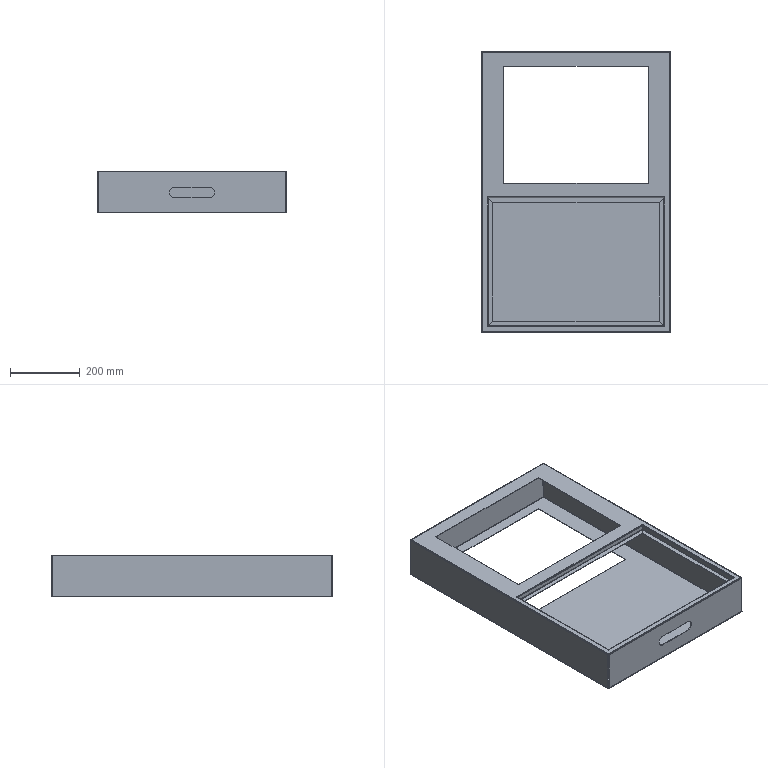Part | STEP file | x77-05301 | 2 solids | 124 faces | box 540 x 803 x 120 mm | volume 1120219 mm3 | plane 74 | cylinder 26 | spline 24 | commonest cylinder face diameters 1.473 x12 4.473 x12 30 x2